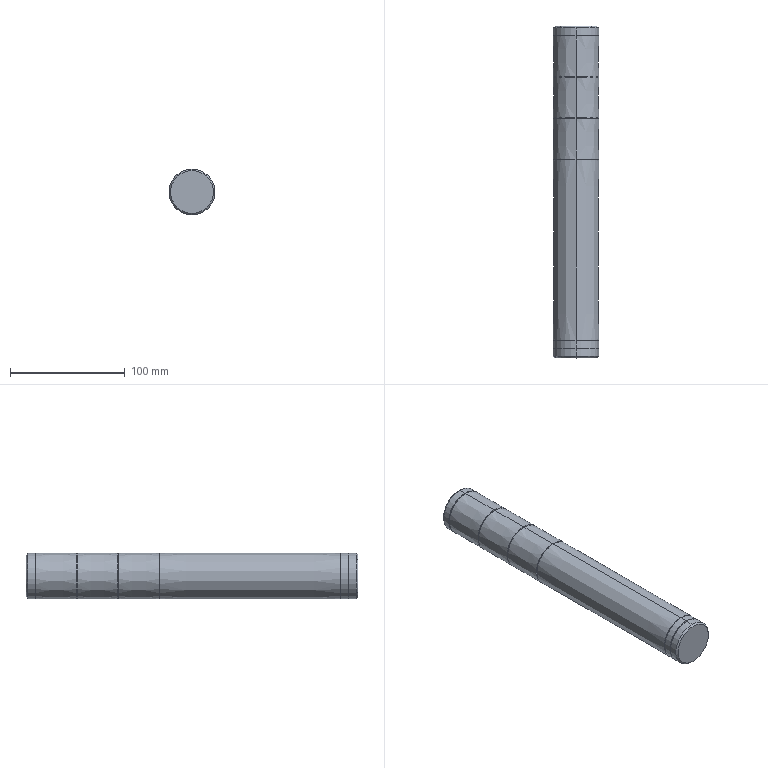Part | STEP file | SceondRR_Default | 1 solid | 46 faces | box 40 x 289 x 40 mm | volume 362543 mm3 | cone 20 | cylinder 14 | plane 12 | commonest cylinder face diameters 38.606 x8 40 x4 39.333 x2